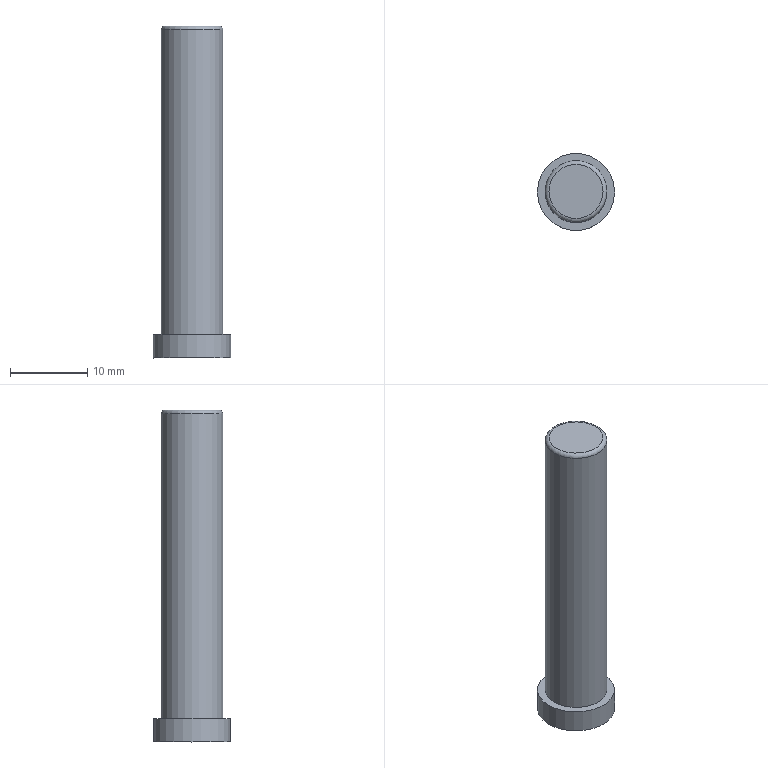Part | NX | features solid 2 | 1 solid | 6 faces | box 10 x 10 x 43 mm | volume 2245 mm3 | plane 3 | cylinder 2 | torus 1 | commonest cylinder face diameters 8 x1 10 x1
STEP:
#1=CARTESIAN_POINT('',(2608.705,270.073,-32.8));
#2=VERTEX_POINT('',#1);
#3=CARTESIAN_POINT('',(2612.205,270.073,-32.8));
#4=DIRECTION('',(0.000000001,0.,-1.));
#5=DIRECTION('',(-1.,0.000000001,-0.000000001));
#6=AXIS2_PLACEMENT_3D('',#3,#4,#5);
#7=CIRCLE('',#6,3.5);
#8=EDGE_CURVE('',#2,#2,#7,.T.);
#9=ORIENTED_EDGE('',*,*,#8,.F.);
#10=EDGE_LOOP('',(#9));
#11=FACE_BOUND('',#10,.T.);
#12=CARTESIAN_POINT('',(2612.205,270.073,-32.8));
#13=DIRECTION('',(-0.000000001,0.,1.));
#14=DIRECTION('',(1.,-0.000000001,0.000000001));
#15=AXIS2_PLACEMENT_3D('',#12,#13,#14);
#16=PLANE('',#15);
#17=ADVANCED_FACE('',(#11),#16,.T.);
#18=CARTESIAN_POINT('',(2608.205,270.073,-72.8));
#19=VERTEX_POINT('',#18);
#20=CARTESIAN_POINT('',(2612.205,270.073,-72.8));
#21=DIRECTION('',(-0.000000001,0.,1.));
#22=DIRECTION('',(-1.,0.000000001,-0.000000001));
#23=AXIS2_PLACEMENT_3D('',#20,#21,#22);
#24=CIRCLE('',#23,4.);
#25=EDGE_CURVE('',#19,#19,#24,.T.);
#26=ORIENTED_EDGE('',*,*,#25,.T.);
#27=EDGE_LOOP('',(#26));
#28=FACE_BOUND('',#27,.T.);
#29=CARTESIAN_POINT('',(2608.205,270.073,-33.3));
#30=VERTEX_POINT('',#29);
#31=CARTESIAN_POINT('',(2612.205,270.073,-33.3));
#32=DIRECTION('',(-0.000000001,0.,1.));
#33=DIRECTION('',(-1.,0.000000001,-0.000000001));
#34=AXIS2_PLACEMENT_3D('',#31,#32,#33);
#35=CIRCLE('',#34,4.);
#36=EDGE_CURVE('',#30,#30,#35,.T.);
#37=ORIENTED_EDGE('',*,*,#36,.F.);
#38=EDGE_LOOP('',(#37));
#39=FACE_BOUND('',#38,.T.);
#40=CARTESIAN_POINT('',(2612.205,270.073,-75.8));
#41=DIRECTION('',(-0.000000001,0.,1.));
#42=DIRECTION('',(1.,-0.000000001,0.000000001));
#43=AXIS2_PLACEMENT_3D('',#40,#41,#42);
#44=CYLINDRICAL_SURFACE('',#43,4.);
#45=ADVANCED_FACE('',(#28,#39),#44,.T.);
#46=ORIENTED_EDGE('',*,*,#8,.T.);
#47=EDGE_LOOP('',(#46));
#48=FACE_BOUND('',#47,.T.);
#49=ORIENTED_EDGE('',*,*,#36,.T.);
#50=EDGE_LOOP('',(#49));
#51=FACE_BOUND('',#50,.T.);
#52=CARTESIAN_POINT('',(2612.205,270.073,-33.3));
#53=DIRECTION('',(-0.000000001,0.,1.));
#54=DIRECTION('',(1.,-0.000000001,0.000000001));
#55=AXIS2_PLACEMENT_3D('',#52,#53,#54);
#56=TOROIDAL_SURFACE('',#55,3.5,0.5);
#57=ADVANCED_FACE('',(#48,#51),#56,.T.);
#58=ORIENTED_EDGE('',*,*,#25,.F.);
#59=EDGE_LOOP('',(#58));
#60=FACE_BOUND('',#59,.T.);
#61=CARTESIAN_POINT('',(2607.205,270.073,-72.8));
#62=VERTEX_POINT('',#61);
#63=CARTESIAN_POINT('',(2612.205,270.073,-72.8));
#64=DIRECTION('',(-0.000000001,0.,1.));
#65=DIRECTION('',(-1.,0.000000001,-0.000000001));
#66=AXIS2_PLACEMENT_3D('',#63,#64,#65);
#67=CIRCLE('',#66,5.);
#68=EDGE_CURVE('',#62,#62,#67,.T.);
#69=ORIENTED_EDGE('',*,*,#68,.T.);
#70=EDGE_LOOP('',(#69));
#71=FACE_BOUND('',#70,.T.);
#72=CARTESIAN_POINT('',(2612.205,270.073,-72.8));
#73=DIRECTION('',(-0.000000001,0.,1.));
#74=DIRECTION('',(1.,-0.000000001,0.000000001));
#75=AXIS2_PLACEMENT_3D('',#72,#73,#74);
#76=PLANE('',#75);
#77=ADVANCED_FACE('',(#60,#71),#76,.T.);
#78=ORIENTED_EDGE('',*,*,#68,.F.);
#79=EDGE_LOOP('',(#78));
#80=FACE_BOUND('',#79,.T.);
#81=CARTESIAN_POINT('',(2607.205,270.073,-75.8));
#82=VERTEX_POINT('',#81);
#83=CARTESIAN_POINT('',(2612.205,270.073,-75.8));
#84=DIRECTION('',(0.000000001,0.,-1.));
#85=DIRECTION('',(-1.,0.000000001,-0.000000001));
#86=AXIS2_PLACEMENT_3D('',#83,#84,#85);
#87=CIRCLE('',#86,5.);
#88=EDGE_CURVE('',#82,#82,#87,.T.);
#89=ORIENTED_EDGE('',*,*,#88,.F.);
#90=EDGE_LOOP('',(#89));
#91=FACE_BOUND('',#90,.T.);
#92=CARTESIAN_POINT('',(2612.205,270.073,-75.8));
#93=DIRECTION('',(-0.000000001,0.,1.));
#94=DIRECTION('',(1.,-0.000000001,0.000000001));
#95=AXIS2_PLACEMENT_3D('',#92,#93,#94);
#96=CYLINDRICAL_SURFACE('',#95,5.);
#97=ADVANCED_FACE('',(#80,#91),#96,.T.);
#98=ORIENTED_EDGE('',*,*,#88,.T.);
#99=EDGE_LOOP('',(#98));
#100=FACE_BOUND('',#99,.T.);
#101=CARTESIAN_POINT('',(2612.205,270.073,-75.8));
#102=DIRECTION('',(0.000000001,0.,-1.));
#103=DIRECTION('',(-1.,0.000000001,-0.000000001));
#104=AXIS2_PLACEMENT_3D('',#101,#102,#103);
#105=PLANE('',#104);
#106=ADVANCED_FACE('',(#100),#105,.T.);
#107=CLOSED_SHELL('',(#17,#45,#57,#77,#97,#106));
#108=MANIFOLD_SOLID_BREP('',#107);
#109=(LENGTH_UNIT()NAMED_UNIT(*)SI_UNIT(.MILLI.,.METRE.));
#110=UNCERTAINTY_MEASURE_WITH_UNIT(LENGTH_MEASURE(0.00001),#109,'','');
#111=(NAMED_UNIT(*)PLANE_ANGLE_UNIT()SI_UNIT($,.RADIAN.));
#112=(NAMED_UNIT(*)SI_UNIT($,.STERADIAN.)SOLID_ANGLE_UNIT());
#113=(GEOMETRIC_REPRESENTATION_CONTEXT(3)GLOBAL_UNCERTAINTY_ASSIGNED_CONTEXT((#110))GLOBAL_UNIT_ASSIGNED_CONTEXT((#109,#111,#112))REPRESENTATION_CONTEXT('',''));
#114=ADVANCED_BREP_SHAPE_REPRESENTATION('',(#108),#113);